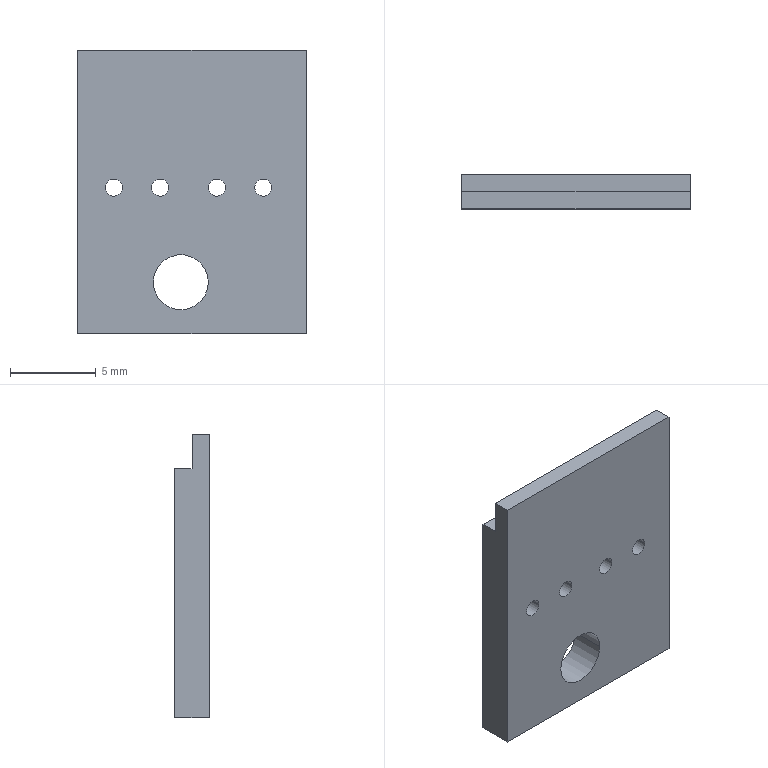Part | STEP file | 06-02-02 light-blocking plate | 1 solid | 18 faces | box 13.3 x 2 x 16.5 mm | volume 389.932 mm3 | cylinder 10 | plane 8 | commonest cylinder face diameters 1 x8 3.2 x2
STEP:
#1=CARTESIAN_POINT('',(-2.25,1.35,5.));
#2=VERTEX_POINT('',#1);
#3=CARTESIAN_POINT('',(0.95,1.35,5.));
#4=VERTEX_POINT('',#3);
#5=CARTESIAN_POINT('',(-0.65,1.35,5.));
#6=DIRECTION('',(0.,-1.,0.));
#7=DIRECTION('',(1.,0.,0.));
#8=AXIS2_PLACEMENT_3D('',#5,#6,#7);
#9=CIRCLE('',#8,1.6);
#10=EDGE_CURVE('',#2,#4,#9,.T.);
#11=ORIENTED_EDGE('',*,*,#10,.F.);
#12=CARTESIAN_POINT('',(-2.25,-0.65,5.));
#13=VERTEX_POINT('',#12);
#14=CARTESIAN_POINT('',(-2.25,9.35,5.));
#15=DIRECTION('',(0.,-1.,0.));
#16=VECTOR('',#15,1000.);
#17=LINE('',#14,#16);
#18=EDGE_CURVE('',#2,#13,#17,.T.);
#19=ORIENTED_EDGE('',*,*,#18,.T.);
#20=CARTESIAN_POINT('',(0.95,-0.65,5.));
#21=VERTEX_POINT('',#20);
#22=CARTESIAN_POINT('',(-0.65,-0.65,5.));
#23=DIRECTION('',(0.,-1.,0.));
#24=DIRECTION('',(1.,0.,0.));
#25=AXIS2_PLACEMENT_3D('',#22,#23,#24);
#26=CIRCLE('',#25,1.6);
#27=EDGE_CURVE('',#13,#21,#26,.T.);
#28=ORIENTED_EDGE('',*,*,#27,.T.);
#29=CARTESIAN_POINT('',(0.95,9.35,5.));
#30=DIRECTION('',(0.,-1.,0.));
#31=VECTOR('',#30,1000.);
#32=LINE('',#29,#31);
#33=EDGE_CURVE('',#4,#21,#32,.T.);
#34=ORIENTED_EDGE('',*,*,#33,.F.);
#35=EDGE_LOOP('',(#11,#19,#28,#34));
#36=FACE_OUTER_BOUND('',#35,.T.);
#37=CARTESIAN_POINT('',(-0.65,9.35,5.));
#38=DIRECTION('',(0.,-1.,0.));
#39=DIRECTION('',(1.,0.,0.));
#40=AXIS2_PLACEMENT_3D('',#37,#38,#39);
#41=CYLINDRICAL_SURFACE('',#40,1.6);
#42=ADVANCED_FACE('',(#36),#41,.F.);
#43=CARTESIAN_POINT('',(3.65,1.35,10.5));
#44=VERTEX_POINT('',#43);
#45=CARTESIAN_POINT('',(4.65,1.35,10.5));
#46=VERTEX_POINT('',#45);
#47=CARTESIAN_POINT('',(4.15,1.35,10.5));
#48=DIRECTION('',(0.,-1.,0.));
#49=DIRECTION('',(1.,0.,0.));
#50=AXIS2_PLACEMENT_3D('',#47,#48,#49);
#51=CIRCLE('',#50,0.5);
#52=EDGE_CURVE('',#44,#46,#51,.T.);
#53=ORIENTED_EDGE('',*,*,#52,.F.);
#54=CARTESIAN_POINT('',(3.65,-0.65,10.5));
#55=VERTEX_POINT('',#54);
#56=CARTESIAN_POINT('',(3.65,9.35,10.5));
#57=DIRECTION('',(0.,-1.,0.));
#58=VECTOR('',#57,1000.);
#59=LINE('',#56,#58);
#60=EDGE_CURVE('',#44,#55,#59,.T.);
#61=ORIENTED_EDGE('',*,*,#60,.T.);
#62=CARTESIAN_POINT('',(4.65,-0.65,10.5));
#63=VERTEX_POINT('',#62);
#64=CARTESIAN_POINT('',(4.15,-0.65,10.5));
#65=DIRECTION('',(0.,-1.,0.));
#66=DIRECTION('',(1.,0.,0.));
#67=AXIS2_PLACEMENT_3D('',#64,#65,#66);
#68=CIRCLE('',#67,0.5);
#69=EDGE_CURVE('',#55,#63,#68,.T.);
#70=ORIENTED_EDGE('',*,*,#69,.T.);
#71=CARTESIAN_POINT('',(4.65,9.35,10.5));
#72=DIRECTION('',(0.,-1.,0.));
#73=VECTOR('',#72,1000.);
#74=LINE('',#71,#73);
#75=EDGE_CURVE('',#46,#63,#74,.T.);
#76=ORIENTED_EDGE('',*,*,#75,.F.);
#77=EDGE_LOOP('',(#53,#61,#70,#76));
#78=FACE_OUTER_BOUND('',#77,.T.);
#79=CARTESIAN_POINT('',(4.15,9.35,10.5));
#80=DIRECTION('',(0.,-1.,0.));
#81=DIRECTION('',(1.,0.,0.));
#82=AXIS2_PLACEMENT_3D('',#79,#80,#81);
#83=CYLINDRICAL_SURFACE('',#82,0.5);
#84=ADVANCED_FACE('',(#78),#83,.F.);
#85=CARTESIAN_POINT('',(0.95,1.35,10.5));
#86=VERTEX_POINT('',#85);
#87=CARTESIAN_POINT('',(1.95,1.35,10.5));
#88=VERTEX_POINT('',#87);
#89=CARTESIAN_POINT('',(1.45,1.35,10.5));
#90=DIRECTION('',(0.,-1.,0.));
#91=DIRECTION('',(1.,0.,0.));
#92=AXIS2_PLACEMENT_3D('',#89,#90,#91);
#93=CIRCLE('',#92,0.5);
#94=EDGE_CURVE('',#86,#88,#93,.T.);
#95=ORIENTED_EDGE('',*,*,#94,.F.);
#96=CARTESIAN_POINT('',(0.95,-0.65,10.5));
#97=VERTEX_POINT('',#96);
#98=CARTESIAN_POINT('',(0.95,9.35,10.5));
#99=DIRECTION('',(0.,-1.,0.));
#100=VECTOR('',#99,1000.);
#101=LINE('',#98,#100);
#102=EDGE_CURVE('',#86,#97,#101,.T.);
#103=ORIENTED_EDGE('',*,*,#102,.T.);
#104=CARTESIAN_POINT('',(1.95,-0.65,10.5));
#105=VERTEX_POINT('',#104);
#106=CARTESIAN_POINT('',(1.45,-0.65,10.5));
#107=DIRECTION('',(0.,-1.,0.));
#108=DIRECTION('',(1.,0.,0.));
#109=AXIS2_PLACEMENT_3D('',#106,#107,#108);
#110=CIRCLE('',#109,0.5);
#111=EDGE_CURVE('',#97,#105,#110,.T.);
#112=ORIENTED_EDGE('',*,*,#111,.T.);
#113=CARTESIAN_POINT('',(1.95,9.35,10.5));
#114=DIRECTION('',(0.,-1.,0.));
#115=VECTOR('',#114,1000.);
#116=LINE('',#113,#115);
#117=EDGE_CURVE('',#88,#105,#116,.T.);
#118=ORIENTED_EDGE('',*,*,#117,.F.);
#119=EDGE_LOOP('',(#95,#103,#112,#118));
#120=FACE_OUTER_BOUND('',#119,.T.);
#121=CARTESIAN_POINT('',(1.45,9.35,10.5));
#122=DIRECTION('',(0.,-1.,0.));
#123=DIRECTION('',(1.,0.,0.));
#124=AXIS2_PLACEMENT_3D('',#121,#122,#123);
#125=CYLINDRICAL_SURFACE('',#124,0.5);
#126=ADVANCED_FACE('',(#120),#125,.F.);
#127=CARTESIAN_POINT('',(-2.35,1.35,10.5));
#128=VERTEX_POINT('',#127);
#129=CARTESIAN_POINT('',(-1.35,1.35,10.5));
#130=VERTEX_POINT('',#129);
#131=CARTESIAN_POINT('',(-1.85,1.35,10.5));
#132=DIRECTION('',(0.,-1.,0.));
#133=DIRECTION('',(1.,0.,0.));
#134=AXIS2_PLACEMENT_3D('',#131,#132,#133);
#135=CIRCLE('',#134,0.5);
#136=EDGE_CURVE('',#128,#130,#135,.T.);
#137=ORIENTED_EDGE('',*,*,#136,.F.);
#138=CARTESIAN_POINT('',(-2.35,-0.65,10.5));
#139=VERTEX_POINT('',#138);
#140=CARTESIAN_POINT('',(-2.35,9.35,10.5));
#141=DIRECTION('',(0.,-1.,0.));
#142=VECTOR('',#141,1000.);
#143=LINE('',#140,#142);
#144=EDGE_CURVE('',#128,#139,#143,.T.);
#145=ORIENTED_EDGE('',*,*,#144,.T.);
#146=CARTESIAN_POINT('',(-1.35,-0.65,10.5));
#147=VERTEX_POINT('',#146);
#148=CARTESIAN_POINT('',(-1.85,-0.65,10.5));
#149=DIRECTION('',(0.,-1.,0.));
#150=DIRECTION('',(1.,0.,0.));
#151=AXIS2_PLACEMENT_3D('',#148,#149,#150);
#152=CIRCLE('',#151,0.5);
#153=EDGE_CURVE('',#139,#147,#152,.T.);
#154=ORIENTED_EDGE('',*,*,#153,.T.);
#155=CARTESIAN_POINT('',(-1.35,9.35,10.5));
#156=DIRECTION('',(0.,-1.,0.));
#157=VECTOR('',#156,1000.);
#158=LINE('',#155,#157);
#159=EDGE_CURVE('',#130,#147,#158,.T.);
#160=ORIENTED_EDGE('',*,*,#159,.F.);
#161=EDGE_LOOP('',(#137,#145,#154,#160));
#162=FACE_OUTER_BOUND('',#161,.T.);
#163=CARTESIAN_POINT('',(-1.85,9.35,10.5));
#164=DIRECTION('',(0.,-1.,0.));
#165=DIRECTION('',(1.,0.,0.));
#166=AXIS2_PLACEMENT_3D('',#163,#164,#165);
#167=CYLINDRICAL_SURFACE('',#166,0.5);
#168=ADVANCED_FACE('',(#162),#167,.F.);
#169=CARTESIAN_POINT('',(-5.05,1.35,10.5));
#170=VERTEX_POINT('',#169);
#171=CARTESIAN_POINT('',(-4.05,1.35,10.5));
#172=VERTEX_POINT('',#171);
#173=CARTESIAN_POINT('',(-4.55,1.35,10.5));
#174=DIRECTION('',(0.,-1.,0.));
#175=DIRECTION('',(1.,0.,0.));
#176=AXIS2_PLACEMENT_3D('',#173,#174,#175);
#177=CIRCLE('',#176,0.5);
#178=EDGE_CURVE('',#170,#172,#177,.T.);
#179=ORIENTED_EDGE('',*,*,#178,.F.);
#180=CARTESIAN_POINT('',(-5.05,-0.65,10.5));
#181=VERTEX_POINT('',#180);
#182=CARTESIAN_POINT('',(-5.05,9.35,10.5));
#183=DIRECTION('',(0.,-1.,0.));
#184=VECTOR('',#183,1000.);
#185=LINE('',#182,#184);
#186=EDGE_CURVE('',#170,#181,#185,.T.);
#187=ORIENTED_EDGE('',*,*,#186,.T.);
#188=CARTESIAN_POINT('',(-4.05,-0.65,10.5));
#189=VERTEX_POINT('',#188);
#190=CARTESIAN_POINT('',(-4.55,-0.65,10.5));
#191=DIRECTION('',(0.,-1.,0.));
#192=DIRECTION('',(1.,0.,0.));
#193=AXIS2_PLACEMENT_3D('',#190,#191,#192);
#194=CIRCLE('',#193,0.5);
#195=EDGE_CURVE('',#181,#189,#194,.T.);
#196=ORIENTED_EDGE('',*,*,#195,.T.);
#197=CARTESIAN_POINT('',(-4.05,9.35,10.5));
#198=DIRECTION('',(0.,-1.,0.));
#199=VECTOR('',#198,1000.);
#200=LINE('',#197,#199);
#201=EDGE_CURVE('',#172,#189,#200,.T.);
#202=ORIENTED_EDGE('',*,*,#201,.F.);
#203=EDGE_LOOP('',(#179,#187,#196,#202));
#204=FACE_OUTER_BOUND('',#203,.T.);
#205=CARTESIAN_POINT('',(-4.55,9.35,10.5));
#206=DIRECTION('',(0.,-1.,0.));
#207=DIRECTION('',(1.,0.,0.));
#208=AXIS2_PLACEMENT_3D('',#205,#206,#207);
#209=CYLINDRICAL_SURFACE('',#208,0.5);
#210=ADVANCED_FACE('',(#204),#209,.F.);
#211=CARTESIAN_POINT('',(6.65,-0.65,18.5));
#212=VERTEX_POINT('',#211);
#213=CARTESIAN_POINT('',(6.65,0.35,18.5));
#214=VERTEX_POINT('',#213);
#215=CARTESIAN_POINT('',(6.65,1.85,18.5));
#216=DIRECTION('',(0.,1.,0.));
#217=VECTOR('',#216,1000.);
#218=LINE('',#215,#217);
#219=EDGE_CURVE('',#212,#214,#218,.T.);
#220=ORIENTED_EDGE('',*,*,#219,.F.);
#221=CARTESIAN_POINT('',(6.65,-0.65,2.));
#222=VERTEX_POINT('',#221);
#223=CARTESIAN_POINT('',(6.65,-0.65,18.998));
#224=DIRECTION('',(0.,0.,1.));
#225=VECTOR('',#224,1000.);
#226=LINE('',#223,#225);
#227=EDGE_CURVE('',#222,#212,#226,.T.);
#228=ORIENTED_EDGE('',*,*,#227,.F.);
#229=CARTESIAN_POINT('',(6.65,1.35,2.));
#230=VERTEX_POINT('',#229);
#231=CARTESIAN_POINT('',(6.65,1.85,2.));
#232=DIRECTION('',(0.,1.,0.));
#233=VECTOR('',#232,1000.);
#234=LINE('',#231,#233);
#235=EDGE_CURVE('',#222,#230,#234,.T.);
#236=ORIENTED_EDGE('',*,*,#235,.T.);
#237=CARTESIAN_POINT('',(6.65,1.35,16.5));
#238=VERTEX_POINT('',#237);
#239=CARTESIAN_POINT('',(6.65,1.35,17.134));
#240=DIRECTION('',(0.,0.,-1.));
#241=VECTOR('',#240,1000.);
#242=LINE('',#239,#241);
#243=EDGE_CURVE('',#238,#230,#242,.T.);
#244=ORIENTED_EDGE('',*,*,#243,.F.);
#245=CARTESIAN_POINT('',(6.65,0.35,16.5));
#246=VERTEX_POINT('',#245);
#247=CARTESIAN_POINT('',(6.65,1.85,16.5));
#248=DIRECTION('',(0.,1.,0.));
#249=VECTOR('',#248,1000.);
#250=LINE('',#247,#249);
#251=EDGE_CURVE('',#246,#238,#250,.T.);
#252=ORIENTED_EDGE('',*,*,#251,.F.);
#253=CARTESIAN_POINT('',(6.65,0.35,18.5));
#254=DIRECTION('',(0.,0.,1.));
#255=VECTOR('',#254,1000.);
#256=LINE('',#253,#255);
#257=EDGE_CURVE('',#246,#214,#256,.T.);
#258=ORIENTED_EDGE('',*,*,#257,.T.);
#259=EDGE_LOOP('',(#220,#228,#236,#244,#252,#258));
#260=FACE_OUTER_BOUND('',#259,.T.);
#261=CARTESIAN_POINT('',(6.65,1.85,18.5));
#262=DIRECTION('',(-1.,0.,0.));
#263=DIRECTION('',(0.,-1.,0.));
#264=AXIS2_PLACEMENT_3D('',#261,#262,#263);
#265=PLANE('',#264);
#266=ADVANCED_FACE('',(#260),#265,.F.);
#267=CARTESIAN_POINT('',(-6.65,-0.65,2.));
#268=VERTEX_POINT('',#267);
#269=CARTESIAN_POINT('',(-6.65,-0.65,18.5));
#270=VERTEX_POINT('',#269);
#271=CARTESIAN_POINT('',(-6.65,-0.65,18.5));
#272=DIRECTION('',(0.,0.,1.));
#273=VECTOR('',#272,1000.);
#274=LINE('',#271,#273);
#275=EDGE_CURVE('',#268,#270,#274,.T.);
#276=ORIENTED_EDGE('',*,*,#275,.T.);
#277=CARTESIAN_POINT('',(-6.65,0.35,18.5));
#278=VERTEX_POINT('',#277);
#279=CARTESIAN_POINT('',(-6.65,1.85,18.5));
#280=DIRECTION('',(0.,-1.,0.));
#281=VECTOR('',#280,1000.);
#282=LINE('',#279,#281);
#283=EDGE_CURVE('',#278,#270,#282,.T.);
#284=ORIENTED_EDGE('',*,*,#283,.F.);
#285=CARTESIAN_POINT('',(-6.65,0.35,16.5));
#286=VERTEX_POINT('',#285);
#287=CARTESIAN_POINT('',(-6.65,0.35,18.5));
#288=DIRECTION('',(0.,0.,-1.));
#289=VECTOR('',#288,1000.);
#290=LINE('',#287,#289);
#291=EDGE_CURVE('',#278,#286,#290,.T.);
#292=ORIENTED_EDGE('',*,*,#291,.T.);
#293=CARTESIAN_POINT('',(-6.65,1.35,16.5));
#294=VERTEX_POINT('',#293);
#295=CARTESIAN_POINT('',(-6.65,1.85,16.5));
#296=DIRECTION('',(0.,-1.,0.));
#297=VECTOR('',#296,1000.);
#298=LINE('',#295,#297);
#299=EDGE_CURVE('',#294,#286,#298,.T.);
#300=ORIENTED_EDGE('',*,*,#299,.F.);
#301=CARTESIAN_POINT('',(-6.65,1.35,2.));
#302=VERTEX_POINT('',#301);
#303=CARTESIAN_POINT('',(-6.65,1.35,18.5));
#304=DIRECTION('',(0.,0.,-1.));
#305=VECTOR('',#304,1000.);
#306=LINE('',#303,#305);
#307=EDGE_CURVE('',#294,#302,#306,.T.);
#308=ORIENTED_EDGE('',*,*,#307,.T.);
#309=CARTESIAN_POINT('',(-6.65,-8.65,2.));
#310=DIRECTION('',(0.,1.,0.));
#311=VECTOR('',#310,1000.);
#312=LINE('',#309,#311);
#313=EDGE_CURVE('',#268,#302,#312,.T.);
#314=ORIENTED_EDGE('',*,*,#313,.F.);
#315=EDGE_LOOP('',(#276,#284,#292,#300,#308,#314));
#316=FACE_OUTER_BOUND('',#315,.T.);
#317=CARTESIAN_POINT('',(-6.65,1.85,18.5));
#318=DIRECTION('',(1.,0.,0.));
#319=DIRECTION('',(0.,1.,0.));
#320=AXIS2_PLACEMENT_3D('',#317,#318,#319);
#321=PLANE('',#320);
#322=ADVANCED_FACE('',(#316),#321,.F.);
#323=ORIENTED_EDGE('',*,*,#283,.T.);
#324=CARTESIAN_POINT('',(6.65,-0.65,18.5));
#325=DIRECTION('',(1.,0.,0.));
#326=VECTOR('',#325,1000.);
#327=LINE('',#324,#326);
#328=EDGE_CURVE('',#270,#212,#327,.T.);
#329=ORIENTED_EDGE('',*,*,#328,.T.);
#330=ORIENTED_EDGE('',*,*,#219,.T.);
#331=CARTESIAN_POINT('',(8.886,0.35,18.5));
#332=DIRECTION('',(-1.,0.,0.));
#333=VECTOR('',#332,1000.);
#334=LINE('',#331,#333);
#335=EDGE_CURVE('',#214,#278,#334,.T.);
#336=ORIENTED_EDGE('',*,*,#335,.T.);
#337=EDGE_LOOP('',(#323,#329,#330,#336));
#338=FACE_OUTER_BOUND('',#337,.T.);
#339=CARTESIAN_POINT('',(6.65,-1.85,18.5));
#340=DIRECTION('',(0.,0.,1.));
#341=DIRECTION('',(1.,0.,0.));
#342=AXIS2_PLACEMENT_3D('',#339,#340,#341);
#343=PLANE('',#342);
#344=ADVANCED_FACE('',(#338),#343,.T.);
#345=CARTESIAN_POINT('',(8.886,0.35,16.5));
#346=DIRECTION('',(-1.,0.,0.));
#347=VECTOR('',#346,1000.);
#348=LINE('',#345,#347);
#349=EDGE_CURVE('',#246,#286,#348,.T.);
#350=ORIENTED_EDGE('',*,*,#349,.F.);
#351=ORIENTED_EDGE('',*,*,#251,.T.);
#352=CARTESIAN_POINT('',(-6.65,1.35,16.5));
#353=DIRECTION('',(1.,0.,0.));
#354=VECTOR('',#353,1000.);
#355=LINE('',#352,#354);
#356=EDGE_CURVE('',#294,#238,#355,.T.);
#357=ORIENTED_EDGE('',*,*,#356,.F.);
#358=ORIENTED_EDGE('',*,*,#299,.T.);
#359=EDGE_LOOP('',(#350,#351,#357,#358));
#360=FACE_OUTER_BOUND('',#359,.T.);
#361=CARTESIAN_POINT('',(-6.65,-0.15,16.5));
#362=DIRECTION('',(0.,0.,1.));
#363=DIRECTION('',(1.,0.,0.));
#364=AXIS2_PLACEMENT_3D('',#361,#362,#363);
#365=PLANE('',#364);
#366=ADVANCED_FACE('',(#360),#365,.T.);
#367=CARTESIAN_POINT('',(-0.65,-0.65,5.));
#368=DIRECTION('',(0.,-1.,0.));
#369=DIRECTION('',(1.,0.,0.));
#370=AXIS2_PLACEMENT_3D('',#367,#368,#369);
#371=CIRCLE('',#370,1.6);
#372=EDGE_CURVE('',#21,#13,#371,.T.);
#373=ORIENTED_EDGE('',*,*,#372,.F.);
#374=ORIENTED_EDGE('',*,*,#27,.F.);
#375=EDGE_LOOP('',(#373,#374));
#376=FACE_BOUND('',#375,.T.);
#377=CARTESIAN_POINT('',(4.15,-0.65,10.5));
#378=DIRECTION('',(0.,-1.,0.));
#379=DIRECTION('',(1.,0.,0.));
#380=AXIS2_PLACEMENT_3D('',#377,#378,#379);
#381=CIRCLE('',#380,0.5);
#382=EDGE_CURVE('',#63,#55,#381,.T.);
#383=ORIENTED_EDGE('',*,*,#382,.F.);
#384=ORIENTED_EDGE('',*,*,#69,.F.);
#385=EDGE_LOOP('',(#383,#384));
#386=FACE_BOUND('',#385,.T.);
#387=CARTESIAN_POINT('',(1.45,-0.65,10.5));
#388=DIRECTION('',(0.,-1.,0.));
#389=DIRECTION('',(1.,0.,0.));
#390=AXIS2_PLACEMENT_3D('',#387,#388,#389);
#391=CIRCLE('',#390,0.5);
#392=EDGE_CURVE('',#105,#97,#391,.T.);
#393=ORIENTED_EDGE('',*,*,#392,.F.);
#394=ORIENTED_EDGE('',*,*,#111,.F.);
#395=EDGE_LOOP('',(#393,#394));
#396=FACE_BOUND('',#395,.T.);
#397=CARTESIAN_POINT('',(-1.85,-0.65,10.5));
#398=DIRECTION('',(0.,-1.,0.));
#399=DIRECTION('',(1.,0.,0.));
#400=AXIS2_PLACEMENT_3D('',#397,#398,#399);
#401=CIRCLE('',#400,0.5);
#402=EDGE_CURVE('',#147,#139,#401,.T.);
#403=ORIENTED_EDGE('',*,*,#402,.F.);
#404=ORIENTED_EDGE('',*,*,#153,.F.);
#405=EDGE_LOOP('',(#403,#404));
#406=FACE_BOUND('',#405,.T.);
#407=CARTESIAN_POINT('',(-4.55,-0.65,10.5));
#408=DIRECTION('',(0.,-1.,0.));
#409=DIRECTION('',(1.,0.,0.));
#410=AXIS2_PLACEMENT_3D('',#407,#408,#409);
#411=CIRCLE('',#410,0.5);
#412=EDGE_CURVE('',#189,#181,#411,.T.);
#413=ORIENTED_EDGE('',*,*,#412,.F.);
#414=ORIENTED_EDGE('',*,*,#195,.F.);
#415=EDGE_LOOP('',(#413,#414));
#416=FACE_BOUND('',#415,.T.);
#417=ORIENTED_EDGE('',*,*,#227,.T.);
#418=ORIENTED_EDGE('',*,*,#328,.F.);
#419=ORIENTED_EDGE('',*,*,#275,.F.);
#420=CARTESIAN_POINT('',(-10.35,-0.65,2.));
#421=DIRECTION('',(1.,0.,0.));
#422=VECTOR('',#421,1000.);
#423=LINE('',#420,#422);
#424=EDGE_CURVE('',#268,#222,#423,.T.);
#425=ORIENTED_EDGE('',*,*,#424,.T.);
#426=EDGE_LOOP('',(#417,#418,#419,#425));
#427=FACE_OUTER_BOUND('',#426,.T.);
#428=CARTESIAN_POINT('',(-10.35,-0.65,18.998));
#429=DIRECTION('',(0.,1.,0.));
#430=DIRECTION('',(-1.,0.,0.));
#431=AXIS2_PLACEMENT_3D('',#428,#429,#430);
#432=PLANE('',#431);
#433=ADVANCED_FACE('',(#376,#386,#396,#406,#416,#427),#432,.F.);
#434=CARTESIAN_POINT('',(-0.65,1.35,5.));
#435=DIRECTION('',(0.,-1.,0.));
#436=DIRECTION('',(1.,0.,0.));
#437=AXIS2_PLACEMENT_3D('',#434,#435,#436);
#438=CIRCLE('',#437,1.6);
#439=EDGE_CURVE('',#4,#2,#438,.T.);
#440=ORIENTED_EDGE('',*,*,#439,.T.);
#441=ORIENTED_EDGE('',*,*,#10,.T.);
#442=EDGE_LOOP('',(#440,#441));
#443=FACE_BOUND('',#442,.T.);
#444=CARTESIAN_POINT('',(4.15,1.35,10.5));
#445=DIRECTION('',(0.,-1.,0.));
#446=DIRECTION('',(1.,0.,0.));
#447=AXIS2_PLACEMENT_3D('',#444,#445,#446);
#448=CIRCLE('',#447,0.5);
#449=EDGE_CURVE('',#46,#44,#448,.T.);
#450=ORIENTED_EDGE('',*,*,#449,.T.);
#451=ORIENTED_EDGE('',*,*,#52,.T.);
#452=EDGE_LOOP('',(#450,#451));
#453=FACE_BOUND('',#452,.T.);
#454=CARTESIAN_POINT('',(1.45,1.35,10.5));
#455=DIRECTION('',(0.,-1.,0.));
#456=DIRECTION('',(1.,0.,0.));
#457=AXIS2_PLACEMENT_3D('',#454,#455,#456);
#458=CIRCLE('',#457,0.5);
#459=EDGE_CURVE('',#88,#86,#458,.T.);
#460=ORIENTED_EDGE('',*,*,#459,.T.);
#461=ORIENTED_EDGE('',*,*,#94,.T.);
#462=EDGE_LOOP('',(#460,#461));
#463=FACE_BOUND('',#462,.T.);
#464=CARTESIAN_POINT('',(-1.85,1.35,10.5));
#465=DIRECTION('',(0.,-1.,0.));
#466=DIRECTION('',(1.,0.,0.));
#467=AXIS2_PLACEMENT_3D('',#464,#465,#466);
#468=CIRCLE('',#467,0.5);
#469=EDGE_CURVE('',#130,#128,#468,.T.);
#470=ORIENTED_EDGE('',*,*,#469,.T.);
#471=ORIENTED_EDGE('',*,*,#136,.T.);
#472=EDGE_LOOP('',(#470,#471));
#473=FACE_BOUND('',#472,.T.);
#474=CARTESIAN_POINT('',(-4.55,1.35,10.5));
#475=DIRECTION('',(0.,-1.,0.));
#476=DIRECTION('',(1.,0.,0.));
#477=AXIS2_PLACEMENT_3D('',#474,#475,#476);
#478=CIRCLE('',#477,0.5);
#479=EDGE_CURVE('',#172,#170,#478,.T.);
#480=ORIENTED_EDGE('',*,*,#479,.T.);
#481=ORIENTED_EDGE('',*,*,#178,.T.);
#482=EDGE_LOOP('',(#480,#481));
#483=FACE_BOUND('',#482,.T.);
#484=ORIENTED_EDGE('',*,*,#243,.T.);
#485=CARTESIAN_POINT('',(-6.65,1.35,2.));
#486=DIRECTION('',(1.,0.,0.));
#487=VECTOR('',#486,1000.);
#488=LINE('',#485,#487);
#489=EDGE_CURVE('',#302,#230,#488,.T.);
#490=ORIENTED_EDGE('',*,*,#489,.F.);
#491=ORIENTED_EDGE('',*,*,#307,.F.);
#492=ORIENTED_EDGE('',*,*,#356,.T.);
#493=EDGE_LOOP('',(#484,#490,#491,#492));
#494=FACE_OUTER_BOUND('',#493,.T.);
#495=CARTESIAN_POINT('',(-10.35,1.35,17.134));
#496=DIRECTION('',(0.,-1.,0.));
#497=DIRECTION('',(1.,0.,0.));
#498=AXIS2_PLACEMENT_3D('',#495,#496,#497);
#499=PLANE('',#498);
#500=ADVANCED_FACE('',(#443,#453,#463,#473,#483,#494),#499,.F.);
#501=ORIENTED_EDGE('',*,*,#424,.F.);
#502=ORIENTED_EDGE('',*,*,#313,.T.);
#503=ORIENTED_EDGE('',*,*,#489,.T.);
#504=ORIENTED_EDGE('',*,*,#235,.F.);
#505=EDGE_LOOP('',(#501,#502,#503,#504));
#506=FACE_OUTER_BOUND('',#505,.T.);
#507=CARTESIAN_POINT('',(-6.65,-8.65,2.));
#508=DIRECTION('',(0.,0.,1.));
#509=DIRECTION('',(1.,0.,0.));
#510=AXIS2_PLACEMENT_3D('',#507,#508,#509);
#511=PLANE('',#510);
#512=ADVANCED_FACE('',(#506),#511,.F.);
#513=ORIENTED_EDGE('',*,*,#186,.F.);
#514=ORIENTED_EDGE('',*,*,#479,.F.);
#515=ORIENTED_EDGE('',*,*,#201,.T.);
#516=ORIENTED_EDGE('',*,*,#412,.T.);
#517=EDGE_LOOP('',(#513,#514,#515,#516));
#518=FACE_OUTER_BOUND('',#517,.T.);
#519=CARTESIAN_POINT('',(-4.55,9.35,10.5));
#520=DIRECTION('',(0.,-1.,0.));
#521=DIRECTION('',(1.,0.,0.));
#522=AXIS2_PLACEMENT_3D('',#519,#520,#521);
#523=CYLINDRICAL_SURFACE('',#522,0.5);
#524=ADVANCED_FACE('',(#518),#523,.F.);
#525=ORIENTED_EDGE('',*,*,#144,.F.);
#526=ORIENTED_EDGE('',*,*,#469,.F.);
#527=ORIENTED_EDGE('',*,*,#159,.T.);
#528=ORIENTED_EDGE('',*,*,#402,.T.);
#529=EDGE_LOOP('',(#525,#526,#527,#528));
#530=FACE_OUTER_BOUND('',#529,.T.);
#531=CARTESIAN_POINT('',(-1.85,9.35,10.5));
#532=DIRECTION('',(0.,-1.,0.));
#533=DIRECTION('',(1.,0.,0.));
#534=AXIS2_PLACEMENT_3D('',#531,#532,#533);
#535=CYLINDRICAL_SURFACE('',#534,0.5);
#536=ADVANCED_FACE('',(#530),#535,.F.);
#537=ORIENTED_EDGE('',*,*,#102,.F.);
#538=ORIENTED_EDGE('',*,*,#459,.F.);
#539=ORIENTED_EDGE('',*,*,#117,.T.);
#540=ORIENTED_EDGE('',*,*,#392,.T.);
#541=EDGE_LOOP('',(#537,#538,#539,#540));
#542=FACE_OUTER_BOUND('',#541,.T.);
#543=CARTESIAN_POINT('',(1.45,9.35,10.5));
#544=DIRECTION('',(0.,-1.,0.));
#545=DIRECTION('',(1.,0.,0.));
#546=AXIS2_PLACEMENT_3D('',#543,#544,#545);
#547=CYLINDRICAL_SURFACE('',#546,0.5);
#548=ADVANCED_FACE('',(#542),#547,.F.);
#549=ORIENTED_EDGE('',*,*,#60,.F.);
#550=ORIENTED_EDGE('',*,*,#449,.F.);
#551=ORIENTED_EDGE('',*,*,#75,.T.);
#552=ORIENTED_EDGE('',*,*,#382,.T.);
#553=EDGE_LOOP('',(#549,#550,#551,#552));
#554=FACE_OUTER_BOUND('',#553,.T.);
#555=CARTESIAN_POINT('',(4.15,9.35,10.5));
#556=DIRECTION('',(0.,-1.,0.));
#557=DIRECTION('',(1.,0.,0.));
#558=AXIS2_PLACEMENT_3D('',#555,#556,#557);
#559=CYLINDRICAL_SURFACE('',#558,0.5);
#560=ADVANCED_FACE('',(#554),#559,.F.);
#561=ORIENTED_EDGE('',*,*,#18,.F.);
#562=ORIENTED_EDGE('',*,*,#439,.F.);
#563=ORIENTED_EDGE('',*,*,#33,.T.);
#564=ORIENTED_EDGE('',*,*,#372,.T.);
#565=EDGE_LOOP('',(#561,#562,#563,#564));
#566=FACE_OUTER_BOUND('',#565,.T.);
#567=CARTESIAN_POINT('',(-0.65,9.35,5.));
#568=DIRECTION('',(0.,-1.,0.));
#569=DIRECTION('',(1.,0.,0.));
#570=AXIS2_PLACEMENT_3D('',#567,#568,#569);
#571=CYLINDRICAL_SURFACE('',#570,1.6);
#572=ADVANCED_FACE('',(#566),#571,.F.);
#573=ORIENTED_EDGE('',*,*,#257,.F.);
#574=ORIENTED_EDGE('',*,*,#349,.T.);
#575=ORIENTED_EDGE('',*,*,#291,.F.);
#576=ORIENTED_EDGE('',*,*,#335,.F.);
#577=EDGE_LOOP('',(#573,#574,#575,#576));
#578=FACE_OUTER_BOUND('',#577,.T.);
#579=CARTESIAN_POINT('',(8.886,0.35,18.5));
#580=DIRECTION('',(0.,1.,0.));
#581=DIRECTION('',(-1.,0.,0.));
#582=AXIS2_PLACEMENT_3D('',#579,#580,#581);
#583=PLANE('',#582);
#584=ADVANCED_FACE('',(#578),#583,.T.);
#585=CLOSED_SHELL('',(#42,#84,#126,#168,#210,#266,#322,#344,#366,#433,#500,#512,#524,#536,#548,#560,#572,#584));
#586=MANIFOLD_SOLID_BREP('',#585);
#587=CARTESIAN_POINT('',(0.,0.,0.));
#588=DIRECTION('',(0.,0.,1.));
#589=DIRECTION('',(1.,0.,0.));
#590=AXIS2_PLACEMENT_3D('',#587,#588,#589);
#591=(LENGTH_UNIT()NAMED_UNIT(*)SI_UNIT(.MILLI.,.METRE.));
#592=UNCERTAINTY_MEASURE_WITH_UNIT(LENGTH_MEASURE(0.00001),#591,'','');
#593=(NAMED_UNIT(*)PLANE_ANGLE_UNIT()SI_UNIT($,.RADIAN.));
#594=(NAMED_UNIT(*)SI_UNIT($,.STERADIAN.)SOLID_ANGLE_UNIT());
#595=(GEOMETRIC_REPRESENTATION_CONTEXT(3)GLOBAL_UNCERTAINTY_ASSIGNED_CONTEXT((#592))GLOBAL_UNIT_ASSIGNED_CONTEXT((#591,#593,#594))REPRESENTATION_CONTEXT('',''));
#596=ADVANCED_BREP_SHAPE_REPRESENTATION('',(#586,#590),#595);